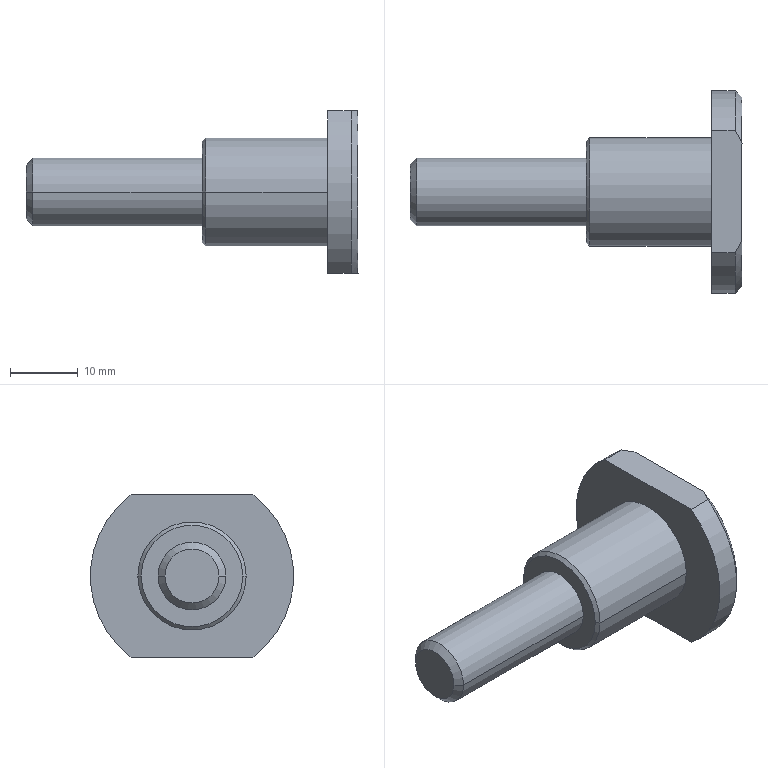Part | STEP file | J306-EBZ05-02-40-Part-1 | 1 solid | 18 faces | box 49 x 30 x 24 mm | volume 8563 mm3 | cone 6 | cylinder 6 | plane 6 | commonest cylinder face diameters 10 x2 16 x2 30 x2
STEP:
#1=CARTESIAN_POINT('',(23.,7.5,0.));
#2=VERTEX_POINT('',#1);
#3=CARTESIAN_POINT('',(23.,-7.5,0.));
#4=VERTEX_POINT('',#3);
#5=CARTESIAN_POINT('',(23.,0.,0.));
#6=DIRECTION('',(-1.,0.,0.));
#7=DIRECTION('',(0.,1.,0.));
#8=AXIS2_PLACEMENT_3D('',#5,#6,#7);
#9=CIRCLE('',#8,7.5);
#10=EDGE_CURVE('',#2,#4,#9,.T.);
#11=ORIENTED_EDGE('',*,*,#10,.F.);
#12=CARTESIAN_POINT('',(23.5,8.,0.));
#13=VERTEX_POINT('',#12);
#14=CARTESIAN_POINT('',(23.5,8.,0.));
#15=DIRECTION('',(0.7071,0.7071,0.));
#16=VECTOR('',#15,1000.);
#17=LINE('',#14,#16);
#18=EDGE_CURVE('',#2,#13,#17,.T.);
#19=ORIENTED_EDGE('',*,*,#18,.T.);
#20=CARTESIAN_POINT('',(23.5,-8.,0.));
#21=VERTEX_POINT('',#20);
#22=CARTESIAN_POINT('',(23.5,0.,0.));
#23=DIRECTION('',(1.,0.,0.));
#24=DIRECTION('',(0.,1.,0.));
#25=AXIS2_PLACEMENT_3D('',#22,#23,#24);
#26=CIRCLE('',#25,8.);
#27=EDGE_CURVE('',#21,#13,#26,.T.);
#28=ORIENTED_EDGE('',*,*,#27,.F.);
#29=CARTESIAN_POINT('',(23.5,-8.,0.));
#30=DIRECTION('',(0.7071,-0.7071,0.));
#31=VECTOR('',#30,1000.);
#32=LINE('',#29,#31);
#33=EDGE_CURVE('',#4,#21,#32,.T.);
#34=ORIENTED_EDGE('',*,*,#33,.F.);
#35=EDGE_LOOP('',(#11,#19,#28,#34));
#36=FACE_OUTER_BOUND('',#35,.T.);
#37=CARTESIAN_POINT('',(23.5,0.,0.));
#38=DIRECTION('',(1.,0.,0.));
#39=DIRECTION('',(0.,-1.,0.));
#40=AXIS2_PLACEMENT_3D('',#37,#38,#39);
#41=CONICAL_SURFACE('',#40,8.,0.7854);
#42=ADVANCED_FACE('',(#36),#41,.T.);
#43=CARTESIAN_POINT('',(-3.,4.,0.));
#44=VERTEX_POINT('',#43);
#45=CARTESIAN_POINT('',(-3.,-4.,0.));
#46=VERTEX_POINT('',#45);
#47=CARTESIAN_POINT('',(-3.,0.,0.));
#48=DIRECTION('',(-1.,0.,0.));
#49=DIRECTION('',(0.,1.,0.));
#50=AXIS2_PLACEMENT_3D('',#47,#48,#49);
#51=CIRCLE('',#50,4.);
#52=EDGE_CURVE('',#44,#46,#51,.T.);
#53=ORIENTED_EDGE('',*,*,#52,.F.);
#54=CARTESIAN_POINT('',(-2.,5.,0.));
#55=VERTEX_POINT('',#54);
#56=CARTESIAN_POINT('',(-2.,5.,0.));
#57=DIRECTION('',(0.7071,0.7071,0.));
#58=VECTOR('',#57,1000.);
#59=LINE('',#56,#58);
#60=EDGE_CURVE('',#44,#55,#59,.T.);
#61=ORIENTED_EDGE('',*,*,#60,.T.);
#62=CARTESIAN_POINT('',(-2.,-5.,0.));
#63=VERTEX_POINT('',#62);
#64=CARTESIAN_POINT('',(-2.,0.,0.));
#65=DIRECTION('',(1.,0.,0.));
#66=DIRECTION('',(0.,1.,0.));
#67=AXIS2_PLACEMENT_3D('',#64,#65,#66);
#68=CIRCLE('',#67,5.);
#69=EDGE_CURVE('',#63,#55,#68,.T.);
#70=ORIENTED_EDGE('',*,*,#69,.F.);
#71=CARTESIAN_POINT('',(-2.,-5.,0.));
#72=DIRECTION('',(0.7071,-0.7071,0.));
#73=VECTOR('',#72,1000.);
#74=LINE('',#71,#73);
#75=EDGE_CURVE('',#46,#63,#74,.T.);
#76=ORIENTED_EDGE('',*,*,#75,.F.);
#77=EDGE_LOOP('',(#53,#61,#70,#76));
#78=FACE_OUTER_BOUND('',#77,.T.);
#79=CARTESIAN_POINT('',(-2.,0.,0.));
#80=DIRECTION('',(1.,0.,0.));
#81=DIRECTION('',(0.,-1.,0.));
#82=AXIS2_PLACEMENT_3D('',#79,#80,#81);
#83=CONICAL_SURFACE('',#82,5.,0.7854);
#84=ADVANCED_FACE('',(#78),#83,.T.);
#85=ORIENTED_EDGE('',*,*,#27,.T.);
#86=CARTESIAN_POINT('',(41.5,8.,0.));
#87=VERTEX_POINT('',#86);
#88=CARTESIAN_POINT('',(23.,8.,0.));
#89=DIRECTION('',(1.,0.,0.));
#90=VECTOR('',#89,1000.);
#91=LINE('',#88,#90);
#92=EDGE_CURVE('',#13,#87,#91,.T.);
#93=ORIENTED_EDGE('',*,*,#92,.T.);
#94=CARTESIAN_POINT('',(41.5,-8.,0.));
#95=VERTEX_POINT('',#94);
#96=CARTESIAN_POINT('',(41.5,0.,0.));
#97=DIRECTION('',(-1.,0.,0.));
#98=DIRECTION('',(0.,1.,0.));
#99=AXIS2_PLACEMENT_3D('',#96,#97,#98);
#100=CIRCLE('',#99,8.);
#101=EDGE_CURVE('',#87,#95,#100,.T.);
#102=ORIENTED_EDGE('',*,*,#101,.T.);
#103=CARTESIAN_POINT('',(23.,-8.,0.));
#104=DIRECTION('',(1.,0.,0.));
#105=VECTOR('',#104,1000.);
#106=LINE('',#103,#105);
#107=EDGE_CURVE('',#21,#95,#106,.T.);
#108=ORIENTED_EDGE('',*,*,#107,.F.);
#109=EDGE_LOOP('',(#85,#93,#102,#108));
#110=FACE_OUTER_BOUND('',#109,.T.);
#111=CARTESIAN_POINT('',(23.,0.,0.));
#112=DIRECTION('',(1.,0.,0.));
#113=DIRECTION('',(0.,-1.,0.));
#114=AXIS2_PLACEMENT_3D('',#111,#112,#113);
#115=CYLINDRICAL_SURFACE('',#114,8.);
#116=ADVANCED_FACE('',(#110),#115,.T.);
#117=ORIENTED_EDGE('',*,*,#69,.T.);
#118=CARTESIAN_POINT('',(23.,5.,0.));
#119=VERTEX_POINT('',#118);
#120=CARTESIAN_POINT('',(-3.,5.,0.));
#121=DIRECTION('',(1.,0.,0.));
#122=VECTOR('',#121,1000.);
#123=LINE('',#120,#122);
#124=EDGE_CURVE('',#55,#119,#123,.T.);
#125=ORIENTED_EDGE('',*,*,#124,.T.);
#126=CARTESIAN_POINT('',(23.,-5.,0.));
#127=VERTEX_POINT('',#126);
#128=CARTESIAN_POINT('',(23.,0.,0.));
#129=DIRECTION('',(-1.,0.,0.));
#130=DIRECTION('',(0.,1.,0.));
#131=AXIS2_PLACEMENT_3D('',#128,#129,#130);
#132=CIRCLE('',#131,5.);
#133=EDGE_CURVE('',#119,#127,#132,.T.);
#134=ORIENTED_EDGE('',*,*,#133,.T.);
#135=CARTESIAN_POINT('',(-3.,-5.,0.));
#136=DIRECTION('',(1.,0.,0.));
#137=VECTOR('',#136,1000.);
#138=LINE('',#135,#137);
#139=EDGE_CURVE('',#63,#127,#138,.T.);
#140=ORIENTED_EDGE('',*,*,#139,.F.);
#141=EDGE_LOOP('',(#117,#125,#134,#140));
#142=FACE_OUTER_BOUND('',#141,.T.);
#143=CARTESIAN_POINT('',(-3.,0.,0.));
#144=DIRECTION('',(1.,0.,0.));
#145=DIRECTION('',(0.,-1.,0.));
#146=AXIS2_PLACEMENT_3D('',#143,#144,#145);
#147=CYLINDRICAL_SURFACE('',#146,5.);
#148=ADVANCED_FACE('',(#142),#147,.T.);
#149=CARTESIAN_POINT('',(46.,7.211,-12.));
#150=VERTEX_POINT('',#149);
#151=CARTESIAN_POINT('',(46.,7.211,12.));
#152=VERTEX_POINT('',#151);
#153=CARTESIAN_POINT('',(46.,0.,0.));
#154=DIRECTION('',(1.,0.,0.));
#155=DIRECTION('',(0.,0.,1.));
#156=AXIS2_PLACEMENT_3D('',#153,#154,#155);
#157=CIRCLE('',#156,14.);
#158=EDGE_CURVE('',#150,#152,#157,.T.);
#159=ORIENTED_EDGE('',*,*,#158,.T.);
#160=CARTESIAN_POINT('',(46.,-7.211,12.));
#161=VERTEX_POINT('',#160);
#162=CARTESIAN_POINT('',(46.,0.,12.));
#163=DIRECTION('',(0.,-1.,0.));
#164=VECTOR('',#163,1000.);
#165=LINE('',#162,#164);
#166=EDGE_CURVE('',#152,#161,#165,.T.);
#167=ORIENTED_EDGE('',*,*,#166,.T.);
#168=CARTESIAN_POINT('',(46.,-7.211,-12.));
#169=VERTEX_POINT('',#168);
#170=CARTESIAN_POINT('',(46.,0.,0.));
#171=DIRECTION('',(1.,0.,0.));
#172=DIRECTION('',(0.,0.,1.));
#173=AXIS2_PLACEMENT_3D('',#170,#171,#172);
#174=CIRCLE('',#173,14.);
#175=EDGE_CURVE('',#161,#169,#174,.T.);
#176=ORIENTED_EDGE('',*,*,#175,.T.);
#177=CARTESIAN_POINT('',(46.,0.,-12.));
#178=DIRECTION('',(0.,1.,0.));
#179=VECTOR('',#178,1000.);
#180=LINE('',#177,#179);
#181=EDGE_CURVE('',#169,#150,#180,.T.);
#182=ORIENTED_EDGE('',*,*,#181,.T.);
#183=EDGE_LOOP('',(#159,#167,#176,#182));
#184=FACE_OUTER_BOUND('',#183,.T.);
#185=CARTESIAN_POINT('',(46.,0.,0.));
#186=DIRECTION('',(1.,0.,0.));
#187=DIRECTION('',(0.,0.,1.));
#188=AXIS2_PLACEMENT_3D('',#185,#186,#187);
#189=PLANE('',#188);
#190=ADVANCED_FACE('',(#184),#189,.T.);
#191=CARTESIAN_POINT('',(41.5,-9.,12.));
#192=VERTEX_POINT('',#191);
#193=CARTESIAN_POINT('',(45.,-9.,12.));
#194=VERTEX_POINT('',#193);
#195=CARTESIAN_POINT('',(46.,-9.,12.));
#196=DIRECTION('',(1.,0.,0.));
#197=VECTOR('',#196,1000.);
#198=LINE('',#195,#197);
#199=EDGE_CURVE('',#192,#194,#198,.T.);
#200=ORIENTED_EDGE('',*,*,#199,.F.);
#201=CARTESIAN_POINT('',(41.5,-9.,-12.));
#202=VERTEX_POINT('',#201);
#203=CARTESIAN_POINT('',(41.5,0.,0.));
#204=DIRECTION('',(1.,0.,0.));
#205=DIRECTION('',(0.,0.,1.));
#206=AXIS2_PLACEMENT_3D('',#203,#204,#205);
#207=CIRCLE('',#206,15.);
#208=EDGE_CURVE('',#192,#202,#207,.T.);
#209=ORIENTED_EDGE('',*,*,#208,.T.);
#210=CARTESIAN_POINT('',(45.,-9.,-12.));
#211=VERTEX_POINT('',#210);
#212=CARTESIAN_POINT('',(46.,-9.,-12.));
#213=DIRECTION('',(-1.,0.,0.));
#214=VECTOR('',#213,1000.);
#215=LINE('',#212,#214);
#216=EDGE_CURVE('',#211,#202,#215,.T.);
#217=ORIENTED_EDGE('',*,*,#216,.F.);
#218=CARTESIAN_POINT('',(45.,0.,0.));
#219=DIRECTION('',(-1.,0.,0.));
#220=DIRECTION('',(0.,0.,1.));
#221=AXIS2_PLACEMENT_3D('',#218,#219,#220);
#222=CIRCLE('',#221,15.);
#223=EDGE_CURVE('',#211,#194,#222,.T.);
#224=ORIENTED_EDGE('',*,*,#223,.T.);
#225=EDGE_LOOP('',(#200,#209,#217,#224));
#226=FACE_OUTER_BOUND('',#225,.T.);
#227=CARTESIAN_POINT('',(46.,0.,0.));
#228=DIRECTION('',(-1.,0.,0.));
#229=DIRECTION('',(0.,0.,-1.));
#230=AXIS2_PLACEMENT_3D('',#227,#228,#229);
#231=CYLINDRICAL_SURFACE('',#230,15.);
#232=ADVANCED_FACE('',(#226),#231,.T.);
#233=CARTESIAN_POINT('',(45.,-9.,12.));
#234=CARTESIAN_POINT('',(45.353,-8.412,12.));
#235=CARTESIAN_POINT('',(45.688,-7.817,12.));
#236=CARTESIAN_POINT('',(46.,-7.211,12.));
#237=B_SPLINE_CURVE_WITH_KNOTS('',3,(#233,#234,#235,#236),.UNSPECIFIED.,.F.,.F.,(4,4),(0.000001351,0.002043),.UNSPECIFIED.);
#238=EDGE_CURVE('',#194,#161,#237,.T.);
#239=ORIENTED_EDGE('',*,*,#238,.F.);
#240=ORIENTED_EDGE('',*,*,#223,.F.);
#241=CARTESIAN_POINT('',(46.,-7.211,-12.));
#242=CARTESIAN_POINT('',(45.687,-7.818,-12.));
#243=CARTESIAN_POINT('',(45.352,-8.413,-12.));
#244=CARTESIAN_POINT('',(45.,-9.,-12.));
#245=B_SPLINE_CURVE_WITH_KNOTS('',3,(#241,#242,#243,#244),.UNSPECIFIED.,.F.,.F.,(4,4),(0.01708,0.01911),.UNSPECIFIED.);
#246=EDGE_CURVE('',#169,#211,#245,.T.);
#247=ORIENTED_EDGE('',*,*,#246,.F.);
#248=ORIENTED_EDGE('',*,*,#175,.F.);
#249=EDGE_LOOP('',(#239,#240,#247,#248));
#250=FACE_OUTER_BOUND('',#249,.T.);
#251=CARTESIAN_POINT('',(45.,0.,0.));
#252=DIRECTION('',(-1.,0.,0.));
#253=DIRECTION('',(0.,0.,-1.));
#254=AXIS2_PLACEMENT_3D('',#251,#252,#253);
#255=CONICAL_SURFACE('',#254,15.,0.7854);
#256=ADVANCED_FACE('',(#250),#255,.T.);
#257=CARTESIAN_POINT('',(41.5,0.,0.));
#258=DIRECTION('',(-1.,0.,0.));
#259=DIRECTION('',(0.,1.,0.));
#260=AXIS2_PLACEMENT_3D('',#257,#258,#259);
#261=CIRCLE('',#260,8.);
#262=EDGE_CURVE('',#95,#87,#261,.T.);
#263=ORIENTED_EDGE('',*,*,#262,.F.);
#264=ORIENTED_EDGE('',*,*,#101,.F.);
#265=EDGE_LOOP('',(#263,#264));
#266=FACE_BOUND('',#265,.T.);
#267=CARTESIAN_POINT('',(41.5,9.,12.));
#268=VERTEX_POINT('',#267);
#269=CARTESIAN_POINT('',(41.5,0.,12.));
#270=DIRECTION('',(0.,-1.,0.));
#271=VECTOR('',#270,1000.);
#272=LINE('',#269,#271);
#273=EDGE_CURVE('',#268,#192,#272,.T.);
#274=ORIENTED_EDGE('',*,*,#273,.F.);
#275=CARTESIAN_POINT('',(41.5,9.,-12.));
#276=VERTEX_POINT('',#275);
#277=CARTESIAN_POINT('',(41.5,0.,0.));
#278=DIRECTION('',(1.,0.,0.));
#279=DIRECTION('',(0.,0.,1.));
#280=AXIS2_PLACEMENT_3D('',#277,#278,#279);
#281=CIRCLE('',#280,15.);
#282=EDGE_CURVE('',#276,#268,#281,.T.);
#283=ORIENTED_EDGE('',*,*,#282,.F.);
#284=CARTESIAN_POINT('',(41.5,0.,-12.));
#285=DIRECTION('',(0.,1.,0.));
#286=VECTOR('',#285,1000.);
#287=LINE('',#284,#286);
#288=EDGE_CURVE('',#202,#276,#287,.T.);
#289=ORIENTED_EDGE('',*,*,#288,.F.);
#290=ORIENTED_EDGE('',*,*,#208,.F.);
#291=EDGE_LOOP('',(#274,#283,#289,#290));
#292=FACE_OUTER_BOUND('',#291,.T.);
#293=CARTESIAN_POINT('',(41.5,0.,0.));
#294=DIRECTION('',(-1.,0.,0.));
#295=DIRECTION('',(0.,0.,-1.));
#296=AXIS2_PLACEMENT_3D('',#293,#294,#295);
#297=PLANE('',#296);
#298=ADVANCED_FACE('',(#266,#292),#297,.T.);
#299=CARTESIAN_POINT('',(45.,9.,12.));
#300=VERTEX_POINT('',#299);
#301=CARTESIAN_POINT('',(46.,9.,12.));
#302=DIRECTION('',(-1.,0.,0.));
#303=VECTOR('',#302,1000.);
#304=LINE('',#301,#303);
#305=EDGE_CURVE('',#300,#268,#304,.T.);
#306=ORIENTED_EDGE('',*,*,#305,.F.);
#307=CARTESIAN_POINT('',(45.,9.,-12.));
#308=VERTEX_POINT('',#307);
#309=CARTESIAN_POINT('',(45.,0.,0.));
#310=DIRECTION('',(-1.,0.,0.));
#311=DIRECTION('',(0.,0.,1.));
#312=AXIS2_PLACEMENT_3D('',#309,#310,#311);
#313=CIRCLE('',#312,15.);
#314=EDGE_CURVE('',#300,#308,#313,.T.);
#315=ORIENTED_EDGE('',*,*,#314,.T.);
#316=CARTESIAN_POINT('',(46.,9.,-12.));
#317=DIRECTION('',(1.,0.,0.));
#318=VECTOR('',#317,1000.);
#319=LINE('',#316,#318);
#320=EDGE_CURVE('',#276,#308,#319,.T.);
#321=ORIENTED_EDGE('',*,*,#320,.F.);
#322=ORIENTED_EDGE('',*,*,#282,.T.);
#323=EDGE_LOOP('',(#306,#315,#321,#322));
#324=FACE_OUTER_BOUND('',#323,.T.);
#325=CARTESIAN_POINT('',(46.,0.,0.));
#326=DIRECTION('',(-1.,0.,0.));
#327=DIRECTION('',(0.,0.,-1.));
#328=AXIS2_PLACEMENT_3D('',#325,#326,#327);
#329=CYLINDRICAL_SURFACE('',#328,15.);
#330=ADVANCED_FACE('',(#324),#329,.T.);
#331=CARTESIAN_POINT('',(46.,7.211,12.));
#332=CARTESIAN_POINT('',(45.687,7.818,12.));
#333=CARTESIAN_POINT('',(45.352,8.413,12.));
#334=CARTESIAN_POINT('',(45.,9.,12.));
#335=B_SPLINE_CURVE_WITH_KNOTS('',3,(#331,#332,#333,#334),.UNSPECIFIED.,.F.,.F.,(4,4),(0.01708,0.01911),.UNSPECIFIED.);
#336=EDGE_CURVE('',#152,#300,#335,.T.);
#337=ORIENTED_EDGE('',*,*,#336,.F.);
#338=ORIENTED_EDGE('',*,*,#158,.F.);
#339=CARTESIAN_POINT('',(45.,9.,-12.));
#340=CARTESIAN_POINT('',(45.353,8.412,-12.));
#341=CARTESIAN_POINT('',(45.688,7.817,-12.));
#342=CARTESIAN_POINT('',(46.,7.211,-12.));
#343=B_SPLINE_CURVE_WITH_KNOTS('',3,(#339,#340,#341,#342),.UNSPECIFIED.,.F.,.F.,(4,4),(0.000001351,0.002043),.UNSPECIFIED.);
#344=EDGE_CURVE('',#308,#150,#343,.T.);
#345=ORIENTED_EDGE('',*,*,#344,.F.);
#346=ORIENTED_EDGE('',*,*,#314,.F.);
#347=EDGE_LOOP('',(#337,#338,#345,#346));
#348=FACE_OUTER_BOUND('',#347,.T.);
#349=CARTESIAN_POINT('',(45.,0.,0.));
#350=DIRECTION('',(-1.,0.,0.));
#351=DIRECTION('',(0.,0.,-1.));
#352=AXIS2_PLACEMENT_3D('',#349,#350,#351);
#353=CONICAL_SURFACE('',#352,15.,0.7854);
#354=ADVANCED_FACE('',(#348),#353,.T.);
#355=ORIENTED_EDGE('',*,*,#344,.T.);
#356=ORIENTED_EDGE('',*,*,#181,.F.);
#357=ORIENTED_EDGE('',*,*,#246,.T.);
#358=ORIENTED_EDGE('',*,*,#216,.T.);
#359=ORIENTED_EDGE('',*,*,#288,.T.);
#360=ORIENTED_EDGE('',*,*,#320,.T.);
#361=EDGE_LOOP('',(#355,#356,#357,#358,#359,#360));
#362=FACE_OUTER_BOUND('',#361,.T.);
#363=CARTESIAN_POINT('',(46.,0.,-12.));
#364=DIRECTION('',(0.,0.,1.));
#365=DIRECTION('',(-1.,0.,0.));
#366=AXIS2_PLACEMENT_3D('',#363,#364,#365);
#367=PLANE('',#366);
#368=ADVANCED_FACE('',(#362),#367,.F.);
#369=ORIENTED_EDGE('',*,*,#238,.T.);
#370=ORIENTED_EDGE('',*,*,#166,.F.);
#371=ORIENTED_EDGE('',*,*,#336,.T.);
#372=ORIENTED_EDGE('',*,*,#305,.T.);
#373=ORIENTED_EDGE('',*,*,#273,.T.);
#374=ORIENTED_EDGE('',*,*,#199,.T.);
#375=EDGE_LOOP('',(#369,#370,#371,#372,#373,#374));
#376=FACE_OUTER_BOUND('',#375,.T.);
#377=CARTESIAN_POINT('',(46.,0.,12.));
#378=DIRECTION('',(0.,0.,-1.));
#379=DIRECTION('',(1.,0.,0.));
#380=AXIS2_PLACEMENT_3D('',#377,#378,#379);
#381=PLANE('',#380);
#382=ADVANCED_FACE('',(#376),#381,.F.);
#383=CARTESIAN_POINT('',(-3.,0.,0.));
#384=DIRECTION('',(-1.,0.,0.));
#385=DIRECTION('',(0.,1.,0.));
#386=AXIS2_PLACEMENT_3D('',#383,#384,#385);
#387=CIRCLE('',#386,4.);
#388=EDGE_CURVE('',#46,#44,#387,.T.);
#389=ORIENTED_EDGE('',*,*,#388,.T.);
#390=ORIENTED_EDGE('',*,*,#52,.T.);
#391=EDGE_LOOP('',(#389,#390));
#392=FACE_OUTER_BOUND('',#391,.T.);
#393=CARTESIAN_POINT('',(-3.,0.,0.));
#394=DIRECTION('',(-1.,0.,0.));
#395=DIRECTION('',(0.,1.,0.));
#396=AXIS2_PLACEMENT_3D('',#393,#394,#395);
#397=PLANE('',#396);
#398=ADVANCED_FACE('',(#392),#397,.T.);
#399=ORIENTED_EDGE('',*,*,#124,.F.);
#400=CARTESIAN_POINT('',(-2.,0.,0.));
#401=DIRECTION('',(1.,0.,0.));
#402=DIRECTION('',(0.,1.,0.));
#403=AXIS2_PLACEMENT_3D('',#400,#401,#402);
#404=CIRCLE('',#403,5.);
#405=EDGE_CURVE('',#55,#63,#404,.T.);
#406=ORIENTED_EDGE('',*,*,#405,.T.);
#407=ORIENTED_EDGE('',*,*,#139,.T.);
#408=CARTESIAN_POINT('',(23.,0.,0.));
#409=DIRECTION('',(-1.,0.,0.));
#410=DIRECTION('',(0.,1.,0.));
#411=AXIS2_PLACEMENT_3D('',#408,#409,#410);
#412=CIRCLE('',#411,5.);
#413=EDGE_CURVE('',#127,#119,#412,.T.);
#414=ORIENTED_EDGE('',*,*,#413,.T.);
#415=EDGE_LOOP('',(#399,#406,#407,#414));
#416=FACE_OUTER_BOUND('',#415,.T.);
#417=CARTESIAN_POINT('',(-3.,0.,0.));
#418=DIRECTION('',(1.,0.,0.));
#419=DIRECTION('',(0.,-1.,0.));
#420=AXIS2_PLACEMENT_3D('',#417,#418,#419);
#421=CYLINDRICAL_SURFACE('',#420,5.);
#422=ADVANCED_FACE('',(#416),#421,.T.);
#423=CARTESIAN_POINT('',(23.,0.,0.));
#424=DIRECTION('',(-1.,0.,0.));
#425=DIRECTION('',(0.,1.,0.));
#426=AXIS2_PLACEMENT_3D('',#423,#424,#425);
#427=CIRCLE('',#426,7.5);
#428=EDGE_CURVE('',#4,#2,#427,.T.);
#429=ORIENTED_EDGE('',*,*,#428,.T.);
#430=ORIENTED_EDGE('',*,*,#10,.T.);
#431=EDGE_LOOP('',(#429,#430));
#432=FACE_OUTER_BOUND('',#431,.T.);
#433=ORIENTED_EDGE('',*,*,#413,.F.);
#434=ORIENTED_EDGE('',*,*,#133,.F.);
#435=EDGE_LOOP('',(#433,#434));
#436=FACE_BOUND('',#435,.T.);
#437=CARTESIAN_POINT('',(23.,0.,0.));
#438=DIRECTION('',(-1.,0.,0.));
#439=DIRECTION('',(0.,1.,0.));
#440=AXIS2_PLACEMENT_3D('',#437,#438,#439);
#441=PLANE('',#440);
#442=ADVANCED_FACE('',(#432,#436),#441,.T.);
#443=ORIENTED_EDGE('',*,*,#92,.F.);
#444=CARTESIAN_POINT('',(23.5,0.,0.));
#445=DIRECTION('',(1.,0.,0.));
#446=DIRECTION('',(0.,1.,0.));
#447=AXIS2_PLACEMENT_3D('',#444,#445,#446);
#448=CIRCLE('',#447,8.);
#449=EDGE_CURVE('',#13,#21,#448,.T.);
#450=ORIENTED_EDGE('',*,*,#449,.T.);
#451=ORIENTED_EDGE('',*,*,#107,.T.);
#452=ORIENTED_EDGE('',*,*,#262,.T.);
#453=EDGE_LOOP('',(#443,#450,#451,#452));
#454=FACE_OUTER_BOUND('',#453,.T.);
#455=CARTESIAN_POINT('',(23.,0.,0.));
#456=DIRECTION('',(1.,0.,0.));
#457=DIRECTION('',(0.,-1.,0.));
#458=AXIS2_PLACEMENT_3D('',#455,#456,#457);
#459=CYLINDRICAL_SURFACE('',#458,8.);
#460=ADVANCED_FACE('',(#454),#459,.T.);
#461=ORIENTED_EDGE('',*,*,#60,.F.);
#462=ORIENTED_EDGE('',*,*,#388,.F.);
#463=ORIENTED_EDGE('',*,*,#75,.T.);
#464=ORIENTED_EDGE('',*,*,#405,.F.);
#465=EDGE_LOOP('',(#461,#462,#463,#464));
#466=FACE_OUTER_BOUND('',#465,.T.);
#467=CARTESIAN_POINT('',(-2.,0.,0.));
#468=DIRECTION('',(1.,0.,0.));
#469=DIRECTION('',(0.,-1.,0.));
#470=AXIS2_PLACEMENT_3D('',#467,#468,#469);
#471=CONICAL_SURFACE('',#470,5.,0.7854);
#472=ADVANCED_FACE('',(#466),#471,.T.);
#473=ORIENTED_EDGE('',*,*,#18,.F.);
#474=ORIENTED_EDGE('',*,*,#428,.F.);
#475=ORIENTED_EDGE('',*,*,#33,.T.);
#476=ORIENTED_EDGE('',*,*,#449,.F.);
#477=EDGE_LOOP('',(#473,#474,#475,#476));
#478=FACE_OUTER_BOUND('',#477,.T.);
#479=CARTESIAN_POINT('',(23.5,0.,0.));
#480=DIRECTION('',(1.,0.,0.));
#481=DIRECTION('',(0.,-1.,0.));
#482=AXIS2_PLACEMENT_3D('',#479,#480,#481);
#483=CONICAL_SURFACE('',#482,8.,0.7854);
#484=ADVANCED_FACE('',(#478),#483,.T.);
#485=CLOSED_SHELL('',(#42,#84,#116,#148,#190,#232,#256,#298,#330,#354,#368,#382,#398,#422,#442,#460,#472,#484));
#486=MANIFOLD_SOLID_BREP('',#485);
#487=CARTESIAN_POINT('',(0.,0.,0.));
#488=DIRECTION('',(0.,0.,1.));
#489=DIRECTION('',(1.,0.,0.));
#490=AXIS2_PLACEMENT_3D('',#487,#488,#489);
#491=(LENGTH_UNIT()NAMED_UNIT(*)SI_UNIT(.MILLI.,.METRE.));
#492=UNCERTAINTY_MEASURE_WITH_UNIT(LENGTH_MEASURE(0.00001),#491,'','');
#493=(NAMED_UNIT(*)PLANE_ANGLE_UNIT()SI_UNIT($,.RADIAN.));
#494=(NAMED_UNIT(*)SI_UNIT($,.STERADIAN.)SOLID_ANGLE_UNIT());
#495=(GEOMETRIC_REPRESENTATION_CONTEXT(3)GLOBAL_UNCERTAINTY_ASSIGNED_CONTEXT((#492))GLOBAL_UNIT_ASSIGNED_CONTEXT((#491,#493,#494))REPRESENTATION_CONTEXT('',''));
#496=ADVANCED_BREP_SHAPE_REPRESENTATION('',(#486,#490),#495);